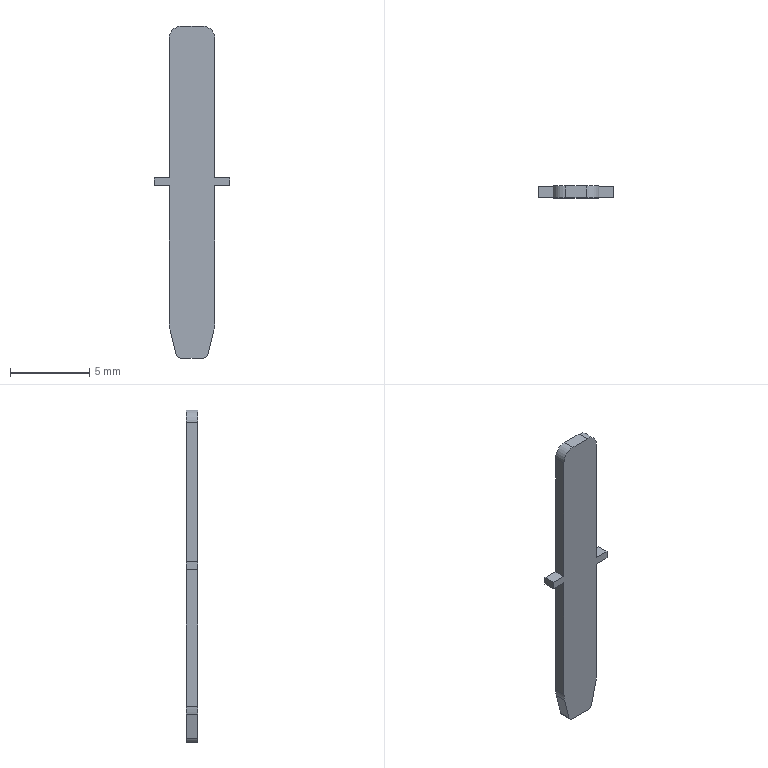Part | SolidWorks | features BaseBody 1 | 1 solid | 22 faces | box 4.8 x 0.75 x 21 mm | volume 45.412 mm3 | plane 16 | cylinder 6 | commonest cylinder face diameters 0.6 x2 1.6 x2 4 x2
STEP:
#1=CARTESIAN_POINT('',(-1.45,0.375,-9.6));
#2=VERTEX_POINT('',#1);
#3=CARTESIAN_POINT('',(-1.45,0.375,-0.8));
#4=VERTEX_POINT('',#3);
#5=CARTESIAN_POINT('',(-1.45,0.375,0.));
#6=DIRECTION('',(0.,0.,1.));
#7=VECTOR('',#6,1000.);
#8=LINE('',#5,#7);
#9=EDGE_CURVE('',#2,#4,#8,.T.);
#10=ORIENTED_EDGE('',*,*,#9,.T.);
#11=CARTESIAN_POINT('',(-0.65,0.375,0.));
#12=VERTEX_POINT('',#11);
#13=CARTESIAN_POINT('',(-0.65,0.375,-0.8));
#14=DIRECTION('',(0.,1.,0.));
#15=DIRECTION('',(0.,0.,-1.));
#16=AXIS2_PLACEMENT_3D('',#13,#14,#15);
#17=CIRCLE('',#16,0.8);
#18=EDGE_CURVE('',#4,#12,#17,.T.);
#19=ORIENTED_EDGE('',*,*,#18,.T.);
#20=CARTESIAN_POINT('',(0.65,0.375,0.));
#21=VERTEX_POINT('',#20);
#22=CARTESIAN_POINT('',(0.,0.375,0.));
#23=DIRECTION('',(1.,0.,0.));
#24=VECTOR('',#23,1000.);
#25=LINE('',#22,#24);
#26=EDGE_CURVE('',#12,#21,#25,.T.);
#27=ORIENTED_EDGE('',*,*,#26,.T.);
#28=CARTESIAN_POINT('',(1.45,0.375,-0.8));
#29=VERTEX_POINT('',#28);
#30=CARTESIAN_POINT('',(0.65,0.375,-0.8));
#31=DIRECTION('',(0.,1.,0.));
#32=DIRECTION('',(0.,0.,-1.));
#33=AXIS2_PLACEMENT_3D('',#30,#31,#32);
#34=CIRCLE('',#33,0.8);
#35=EDGE_CURVE('',#21,#29,#34,.T.);
#36=ORIENTED_EDGE('',*,*,#35,.T.);
#37=CARTESIAN_POINT('',(1.45,0.375,-9.6));
#38=VERTEX_POINT('',#37);
#39=CARTESIAN_POINT('',(1.45,0.375,0.));
#40=DIRECTION('',(0.,0.,-1.));
#41=VECTOR('',#40,1000.);
#42=LINE('',#39,#41);
#43=EDGE_CURVE('',#29,#38,#42,.T.);
#44=ORIENTED_EDGE('',*,*,#43,.T.);
#45=CARTESIAN_POINT('',(2.4,0.375,-9.6));
#46=VERTEX_POINT('',#45);
#47=CARTESIAN_POINT('',(0.,0.375,-9.6));
#48=DIRECTION('',(1.,0.,0.));
#49=VECTOR('',#48,1000.);
#50=LINE('',#47,#49);
#51=EDGE_CURVE('',#38,#46,#50,.T.);
#52=ORIENTED_EDGE('',*,*,#51,.T.);
#53=CARTESIAN_POINT('',(2.4,0.375,-10.1));
#54=VERTEX_POINT('',#53);
#55=CARTESIAN_POINT('',(2.4,0.375,0.));
#56=DIRECTION('',(0.,0.,-1.));
#57=VECTOR('',#56,1000.);
#58=LINE('',#55,#57);
#59=EDGE_CURVE('',#46,#54,#58,.T.);
#60=ORIENTED_EDGE('',*,*,#59,.T.);
#61=CARTESIAN_POINT('',(1.45,0.375,-10.1));
#62=VERTEX_POINT('',#61);
#63=CARTESIAN_POINT('',(0.,0.375,-10.1));
#64=DIRECTION('',(-1.,0.,0.));
#65=VECTOR('',#64,1000.);
#66=LINE('',#63,#65);
#67=EDGE_CURVE('',#54,#62,#66,.T.);
#68=ORIENTED_EDGE('',*,*,#67,.T.);
#69=CARTESIAN_POINT('',(1.45,0.375,-18.754));
#70=VERTEX_POINT('',#69);
#71=CARTESIAN_POINT('',(1.45,0.375,0.));
#72=DIRECTION('',(0.,0.,-1.));
#73=VECTOR('',#72,1000.);
#74=LINE('',#71,#73);
#75=EDGE_CURVE('',#62,#70,#74,.T.);
#76=ORIENTED_EDGE('',*,*,#75,.T.);
#77=CARTESIAN_POINT('',(1.39,0.375,-19.239));
#78=VERTEX_POINT('',#77);
#79=CARTESIAN_POINT('',(-0.55,0.375,-18.754));
#80=DIRECTION('',(0.,1.,0.));
#81=DIRECTION('',(0.,0.,1.));
#82=AXIS2_PLACEMENT_3D('',#79,#80,#81);
#83=CIRCLE('',#82,2.);
#84=EDGE_CURVE('',#70,#78,#83,.T.);
#85=ORIENTED_EDGE('',*,*,#84,.T.);
#86=CARTESIAN_POINT('',(1.007,0.375,-20.773));
#87=VERTEX_POINT('',#86);
#88=CARTESIAN_POINT('',(1.39,0.375,-19.239));
#89=DIRECTION('',(-0.2425,0.,-0.9701));
#90=VECTOR('',#89,1000.);
#91=LINE('',#88,#90);
#92=EDGE_CURVE('',#78,#87,#91,.T.);
#93=ORIENTED_EDGE('',*,*,#92,.T.);
#94=CARTESIAN_POINT('',(0.7158,0.375,-21.));
#95=VERTEX_POINT('',#94);
#96=CARTESIAN_POINT('',(0.7158,0.375,-20.7));
#97=DIRECTION('',(0.,1.,0.));
#98=DIRECTION('',(0.,0.,-1.));
#99=AXIS2_PLACEMENT_3D('',#96,#97,#98);
#100=CIRCLE('',#99,0.3);
#101=EDGE_CURVE('',#87,#95,#100,.T.);
#102=ORIENTED_EDGE('',*,*,#101,.T.);
#103=CARTESIAN_POINT('',(-0.7158,0.375,-21.));
#104=VERTEX_POINT('',#103);
#105=CARTESIAN_POINT('',(0.,0.375,-21.));
#106=DIRECTION('',(-1.,0.,0.));
#107=VECTOR('',#106,1000.);
#108=LINE('',#105,#107);
#109=EDGE_CURVE('',#95,#104,#108,.T.);
#110=ORIENTED_EDGE('',*,*,#109,.T.);
#111=CARTESIAN_POINT('',(-1.007,0.375,-20.773));
#112=VERTEX_POINT('',#111);
#113=CARTESIAN_POINT('',(-0.7158,0.375,-20.7));
#114=DIRECTION('',(0.,1.,0.));
#115=DIRECTION('',(0.,0.,1.));
#116=AXIS2_PLACEMENT_3D('',#113,#114,#115);
#117=CIRCLE('',#116,0.3);
#118=EDGE_CURVE('',#104,#112,#117,.T.);
#119=ORIENTED_EDGE('',*,*,#118,.T.);
#120=CARTESIAN_POINT('',(-1.39,0.375,-19.239));
#121=VERTEX_POINT('',#120);
#122=CARTESIAN_POINT('',(-1.007,0.375,-20.773));
#123=DIRECTION('',(-0.2425,0.,0.9701));
#124=VECTOR('',#123,1000.);
#125=LINE('',#122,#124);
#126=EDGE_CURVE('',#112,#121,#125,.T.);
#127=ORIENTED_EDGE('',*,*,#126,.T.);
#128=CARTESIAN_POINT('',(-1.45,0.375,-18.754));
#129=VERTEX_POINT('',#128);
#130=CARTESIAN_POINT('',(0.55,0.375,-18.754));
#131=DIRECTION('',(0.,1.,0.));
#132=DIRECTION('',(0.,0.,-1.));
#133=AXIS2_PLACEMENT_3D('',#130,#131,#132);
#134=CIRCLE('',#133,2.);
#135=EDGE_CURVE('',#121,#129,#134,.T.);
#136=ORIENTED_EDGE('',*,*,#135,.T.);
#137=CARTESIAN_POINT('',(-1.45,0.375,-10.1));
#138=VERTEX_POINT('',#137);
#139=CARTESIAN_POINT('',(-1.45,0.375,0.));
#140=DIRECTION('',(0.,0.,1.));
#141=VECTOR('',#140,1000.);
#142=LINE('',#139,#141);
#143=EDGE_CURVE('',#129,#138,#142,.T.);
#144=ORIENTED_EDGE('',*,*,#143,.T.);
#145=CARTESIAN_POINT('',(-2.4,0.375,-10.1));
#146=VERTEX_POINT('',#145);
#147=CARTESIAN_POINT('',(0.,0.375,-10.1));
#148=DIRECTION('',(-1.,0.,0.));
#149=VECTOR('',#148,1000.);
#150=LINE('',#147,#149);
#151=EDGE_CURVE('',#138,#146,#150,.T.);
#152=ORIENTED_EDGE('',*,*,#151,.T.);
#153=CARTESIAN_POINT('',(-2.4,0.375,-9.6));
#154=VERTEX_POINT('',#153);
#155=CARTESIAN_POINT('',(-2.4,0.375,0.));
#156=DIRECTION('',(0.,0.,1.));
#157=VECTOR('',#156,1000.);
#158=LINE('',#155,#157);
#159=EDGE_CURVE('',#146,#154,#158,.T.);
#160=ORIENTED_EDGE('',*,*,#159,.T.);
#161=CARTESIAN_POINT('',(0.,0.375,-9.6));
#162=DIRECTION('',(1.,0.,0.));
#163=VECTOR('',#162,1000.);
#164=LINE('',#161,#163);
#165=EDGE_CURVE('',#154,#2,#164,.T.);
#166=ORIENTED_EDGE('',*,*,#165,.T.);
#167=EDGE_LOOP('',(#10,#19,#27,#36,#44,#52,#60,#68,#76,#85,#93,#102,#110,#119,#127,#136,#144,#152,#160,#166));
#168=FACE_OUTER_BOUND('',#167,.T.);
#169=CARTESIAN_POINT('',(0.,0.375,0.));
#170=DIRECTION('',(0.,1.,0.));
#171=DIRECTION('',(0.,0.,1.));
#172=AXIS2_PLACEMENT_3D('',#169,#170,#171);
#173=PLANE('',#172);
#174=ADVANCED_FACE('',(#168),#173,.T.);
#175=CARTESIAN_POINT('',(-1.45,-0.375,-0.8));
#176=VERTEX_POINT('',#175);
#177=CARTESIAN_POINT('',(-1.45,1.413,-0.8));
#178=DIRECTION('',(0.,-1.,0.));
#179=VECTOR('',#178,1000.);
#180=LINE('',#177,#179);
#181=EDGE_CURVE('',#4,#176,#180,.T.);
#182=ORIENTED_EDGE('',*,*,#181,.T.);
#183=CARTESIAN_POINT('',(-0.65,-0.375,0.));
#184=VERTEX_POINT('',#183);
#185=CARTESIAN_POINT('',(-0.65,-0.375,-0.8));
#186=DIRECTION('',(0.,1.,0.));
#187=DIRECTION('',(0.,0.,-1.));
#188=AXIS2_PLACEMENT_3D('',#185,#186,#187);
#189=CIRCLE('',#188,0.8);
#190=EDGE_CURVE('',#176,#184,#189,.T.);
#191=ORIENTED_EDGE('',*,*,#190,.T.);
#192=CARTESIAN_POINT('',(-0.65,1.413,0.));
#193=DIRECTION('',(0.,1.,0.));
#194=VECTOR('',#193,1000.);
#195=LINE('',#192,#194);
#196=EDGE_CURVE('',#184,#12,#195,.T.);
#197=ORIENTED_EDGE('',*,*,#196,.T.);
#198=ORIENTED_EDGE('',*,*,#18,.F.);
#199=EDGE_LOOP('',(#182,#191,#197,#198));
#200=FACE_OUTER_BOUND('',#199,.T.);
#201=CARTESIAN_POINT('',(-0.65,1.413,-0.8));
#202=DIRECTION('',(0.,-1.,0.));
#203=DIRECTION('',(0.,0.,-1.));
#204=AXIS2_PLACEMENT_3D('',#201,#202,#203);
#205=CYLINDRICAL_SURFACE('',#204,0.8);
#206=ADVANCED_FACE('',(#200),#205,.T.);
#207=CARTESIAN_POINT('',(-1.45,-0.375,-9.6));
#208=VERTEX_POINT('',#207);
#209=CARTESIAN_POINT('',(-1.45,-0.375,-21.));
#210=DIRECTION('',(0.,0.,1.));
#211=VECTOR('',#210,1000.);
#212=LINE('',#209,#211);
#213=EDGE_CURVE('',#208,#176,#212,.T.);
#214=ORIENTED_EDGE('',*,*,#213,.T.);
#215=ORIENTED_EDGE('',*,*,#181,.F.);
#216=ORIENTED_EDGE('',*,*,#9,.F.);
#217=CARTESIAN_POINT('',(-1.45,-0.375,-9.6));
#218=DIRECTION('',(0.,-1.,0.));
#219=VECTOR('',#218,1000.);
#220=LINE('',#217,#219);
#221=EDGE_CURVE('',#2,#208,#220,.T.);
#222=ORIENTED_EDGE('',*,*,#221,.T.);
#223=EDGE_LOOP('',(#214,#215,#216,#222));
#224=FACE_OUTER_BOUND('',#223,.T.);
#225=CARTESIAN_POINT('',(-1.45,-0.375,-21.));
#226=DIRECTION('',(-1.,0.,0.));
#227=DIRECTION('',(0.,0.,1.));
#228=AXIS2_PLACEMENT_3D('',#225,#226,#227);
#229=PLANE('',#228);
#230=ADVANCED_FACE('',(#224),#229,.T.);
#231=CARTESIAN_POINT('',(-2.4,-0.375,-9.6));
#232=VERTEX_POINT('',#231);
#233=CARTESIAN_POINT('',(-2.4,-0.375,-9.6));
#234=DIRECTION('',(1.,0.,0.));
#235=VECTOR('',#234,1000.);
#236=LINE('',#233,#235);
#237=EDGE_CURVE('',#232,#208,#236,.T.);
#238=ORIENTED_EDGE('',*,*,#237,.T.);
#239=ORIENTED_EDGE('',*,*,#221,.F.);
#240=ORIENTED_EDGE('',*,*,#165,.F.);
#241=CARTESIAN_POINT('',(-2.4,0.375,-9.6));
#242=DIRECTION('',(0.,-1.,0.));
#243=VECTOR('',#242,1000.);
#244=LINE('',#241,#243);
#245=EDGE_CURVE('',#154,#232,#244,.T.);
#246=ORIENTED_EDGE('',*,*,#245,.T.);
#247=EDGE_LOOP('',(#238,#239,#240,#246));
#248=FACE_OUTER_BOUND('',#247,.T.);
#249=CARTESIAN_POINT('',(-2.4,0.375,-9.6));
#250=DIRECTION('',(0.,0.,1.));
#251=DIRECTION('',(1.,0.,0.));
#252=AXIS2_PLACEMENT_3D('',#249,#250,#251);
#253=PLANE('',#252);
#254=ADVANCED_FACE('',(#248),#253,.T.);
#255=ORIENTED_EDGE('',*,*,#245,.F.);
#256=ORIENTED_EDGE('',*,*,#159,.F.);
#257=CARTESIAN_POINT('',(-2.4,-0.375,-10.1));
#258=VERTEX_POINT('',#257);
#259=CARTESIAN_POINT('',(-2.4,0.375,-10.1));
#260=DIRECTION('',(0.,-1.,0.));
#261=VECTOR('',#260,1000.);
#262=LINE('',#259,#261);
#263=EDGE_CURVE('',#146,#258,#262,.T.);
#264=ORIENTED_EDGE('',*,*,#263,.T.);
#265=CARTESIAN_POINT('',(-2.4,-0.375,-10.1));
#266=DIRECTION('',(0.,0.,1.));
#267=VECTOR('',#266,1000.);
#268=LINE('',#265,#267);
#269=EDGE_CURVE('',#258,#232,#268,.T.);
#270=ORIENTED_EDGE('',*,*,#269,.T.);
#271=EDGE_LOOP('',(#255,#256,#264,#270));
#272=FACE_OUTER_BOUND('',#271,.T.);
#273=CARTESIAN_POINT('',(-2.4,0.375,-10.1));
#274=DIRECTION('',(-1.,0.,0.));
#275=DIRECTION('',(0.,0.,1.));
#276=AXIS2_PLACEMENT_3D('',#273,#274,#275);
#277=PLANE('',#276);
#278=ADVANCED_FACE('',(#272),#277,.T.);
#279=ORIENTED_EDGE('',*,*,#151,.F.);
#280=CARTESIAN_POINT('',(-1.45,-0.375,-10.1));
#281=VERTEX_POINT('',#280);
#282=CARTESIAN_POINT('',(-1.45,0.375,-10.1));
#283=DIRECTION('',(0.,-1.,0.));
#284=VECTOR('',#283,1000.);
#285=LINE('',#282,#284);
#286=EDGE_CURVE('',#138,#281,#285,.T.);
#287=ORIENTED_EDGE('',*,*,#286,.T.);
#288=CARTESIAN_POINT('',(2.4,-0.375,-10.1));
#289=DIRECTION('',(-1.,0.,0.));
#290=VECTOR('',#289,1000.);
#291=LINE('',#288,#290);
#292=EDGE_CURVE('',#281,#258,#291,.T.);
#293=ORIENTED_EDGE('',*,*,#292,.T.);
#294=ORIENTED_EDGE('',*,*,#263,.F.);
#295=EDGE_LOOP('',(#279,#287,#293,#294));
#296=FACE_OUTER_BOUND('',#295,.T.);
#297=CARTESIAN_POINT('',(2.4,0.375,-10.1));
#298=DIRECTION('',(0.,0.,-1.));
#299=DIRECTION('',(-1.,0.,0.));
#300=AXIS2_PLACEMENT_3D('',#297,#298,#299);
#301=PLANE('',#300);
#302=ADVANCED_FACE('',(#296),#301,.T.);
#303=ORIENTED_EDGE('',*,*,#143,.F.);
#304=CARTESIAN_POINT('',(-1.45,-0.375,-18.754));
#305=VERTEX_POINT('',#304);
#306=CARTESIAN_POINT('',(-1.45,-0.375,-18.754));
#307=DIRECTION('',(0.,-1.,0.));
#308=VECTOR('',#307,1000.);
#309=LINE('',#306,#308);
#310=EDGE_CURVE('',#129,#305,#309,.T.);
#311=ORIENTED_EDGE('',*,*,#310,.T.);
#312=CARTESIAN_POINT('',(-1.45,-0.375,-21.));
#313=DIRECTION('',(0.,0.,1.));
#314=VECTOR('',#313,1000.);
#315=LINE('',#312,#314);
#316=EDGE_CURVE('',#305,#281,#315,.T.);
#317=ORIENTED_EDGE('',*,*,#316,.T.);
#318=ORIENTED_EDGE('',*,*,#286,.F.);
#319=EDGE_LOOP('',(#303,#311,#317,#318));
#320=FACE_OUTER_BOUND('',#319,.T.);
#321=CARTESIAN_POINT('',(-1.45,-0.375,-21.));
#322=DIRECTION('',(-1.,0.,0.));
#323=DIRECTION('',(0.,0.,1.));
#324=AXIS2_PLACEMENT_3D('',#321,#322,#323);
#325=PLANE('',#324);
#326=ADVANCED_FACE('',(#320),#325,.T.);
#327=CARTESIAN_POINT('',(-1.39,-0.375,-19.239));
#328=VERTEX_POINT('',#327);
#329=CARTESIAN_POINT('',(-1.39,2.856,-19.239));
#330=DIRECTION('',(0.,-1.,0.));
#331=VECTOR('',#330,1000.);
#332=LINE('',#329,#331);
#333=EDGE_CURVE('',#121,#328,#332,.T.);
#334=ORIENTED_EDGE('',*,*,#333,.T.);
#335=CARTESIAN_POINT('',(0.55,-0.375,-18.754));
#336=DIRECTION('',(0.,1.,0.));
#337=DIRECTION('',(0.,0.,-1.));
#338=AXIS2_PLACEMENT_3D('',#335,#336,#337);
#339=CIRCLE('',#338,2.);
#340=EDGE_CURVE('',#328,#305,#339,.T.);
#341=ORIENTED_EDGE('',*,*,#340,.T.);
#342=ORIENTED_EDGE('',*,*,#310,.F.);
#343=ORIENTED_EDGE('',*,*,#135,.F.);
#344=EDGE_LOOP('',(#334,#341,#342,#343));
#345=FACE_OUTER_BOUND('',#344,.T.);
#346=CARTESIAN_POINT('',(0.55,2.856,-18.754));
#347=DIRECTION('',(0.,-1.,0.));
#348=DIRECTION('',(0.,0.,-1.));
#349=AXIS2_PLACEMENT_3D('',#346,#347,#348);
#350=CYLINDRICAL_SURFACE('',#349,2.);
#351=ADVANCED_FACE('',(#345),#350,.T.);
#352=ORIENTED_EDGE('',*,*,#126,.F.);
#353=CARTESIAN_POINT('',(-1.007,-0.375,-20.773));
#354=VERTEX_POINT('',#353);
#355=CARTESIAN_POINT('',(-1.007,0.,-20.773));
#356=DIRECTION('',(0.,-1.,0.));
#357=VECTOR('',#356,1000.);
#358=LINE('',#355,#357);
#359=EDGE_CURVE('',#112,#354,#358,.T.);
#360=ORIENTED_EDGE('',*,*,#359,.T.);
#361=CARTESIAN_POINT('',(-1.2,-0.375,-20.));
#362=DIRECTION('',(-0.2425,0.,0.9701));
#363=VECTOR('',#362,1000.);
#364=LINE('',#361,#363);
#365=EDGE_CURVE('',#354,#328,#364,.T.);
#366=ORIENTED_EDGE('',*,*,#365,.T.);
#367=ORIENTED_EDGE('',*,*,#333,.F.);
#368=EDGE_LOOP('',(#352,#360,#366,#367));
#369=FACE_OUTER_BOUND('',#368,.T.);
#370=CARTESIAN_POINT('',(-1.2,0.,-20.));
#371=DIRECTION('',(-0.9701,0.,-0.2425));
#372=DIRECTION('',(-0.2425,0.,0.9701));
#373=AXIS2_PLACEMENT_3D('',#370,#371,#372);
#374=PLANE('',#373);
#375=ADVANCED_FACE('',(#369),#374,.T.);
#376=ORIENTED_EDGE('',*,*,#359,.F.);
#377=ORIENTED_EDGE('',*,*,#118,.F.);
#378=CARTESIAN_POINT('',(-0.7158,-0.375,-21.));
#379=VERTEX_POINT('',#378);
#380=CARTESIAN_POINT('',(-0.7158,-1.353,-21.));
#381=DIRECTION('',(0.,-1.,0.));
#382=VECTOR('',#381,1000.);
#383=LINE('',#380,#382);
#384=EDGE_CURVE('',#104,#379,#383,.T.);
#385=ORIENTED_EDGE('',*,*,#384,.T.);
#386=CARTESIAN_POINT('',(-0.7158,-0.375,-20.7));
#387=DIRECTION('',(0.,1.,0.));
#388=DIRECTION('',(0.,0.,1.));
#389=AXIS2_PLACEMENT_3D('',#386,#387,#388);
#390=CIRCLE('',#389,0.3);
#391=EDGE_CURVE('',#379,#354,#390,.T.);
#392=ORIENTED_EDGE('',*,*,#391,.T.);
#393=EDGE_LOOP('',(#376,#377,#385,#392));
#394=FACE_OUTER_BOUND('',#393,.T.);
#395=CARTESIAN_POINT('',(-0.7158,-1.353,-20.7));
#396=DIRECTION('',(0.,1.,0.));
#397=DIRECTION('',(0.,0.,1.));
#398=AXIS2_PLACEMENT_3D('',#395,#396,#397);
#399=CYLINDRICAL_SURFACE('',#398,0.3);
#400=ADVANCED_FACE('',(#394),#399,.T.);
#401=ORIENTED_EDGE('',*,*,#109,.F.);
#402=CARTESIAN_POINT('',(0.7158,-0.375,-21.));
#403=VERTEX_POINT('',#402);
#404=CARTESIAN_POINT('',(0.7158,-0.375,-21.));
#405=DIRECTION('',(0.,-1.,0.));
#406=VECTOR('',#405,1000.);
#407=LINE('',#404,#406);
#408=EDGE_CURVE('',#95,#403,#407,.T.);
#409=ORIENTED_EDGE('',*,*,#408,.T.);
#410=CARTESIAN_POINT('',(1.45,-0.375,-21.));
#411=DIRECTION('',(-1.,0.,0.));
#412=VECTOR('',#411,1000.);
#413=LINE('',#410,#412);
#414=EDGE_CURVE('',#403,#379,#413,.T.);
#415=ORIENTED_EDGE('',*,*,#414,.T.);
#416=ORIENTED_EDGE('',*,*,#384,.F.);
#417=EDGE_LOOP('',(#401,#409,#415,#416));
#418=FACE_OUTER_BOUND('',#417,.T.);
#419=CARTESIAN_POINT('',(1.45,-0.375,-21.));
#420=DIRECTION('',(0.,0.,-1.));
#421=DIRECTION('',(-1.,0.,0.));
#422=AXIS2_PLACEMENT_3D('',#419,#420,#421);
#423=PLANE('',#422);
#424=ADVANCED_FACE('',(#418),#423,.T.);
#425=CARTESIAN_POINT('',(1.007,-0.375,-20.773));
#426=VERTEX_POINT('',#425);
#427=CARTESIAN_POINT('',(1.007,1.353,-20.773));
#428=DIRECTION('',(0.,-1.,0.));
#429=VECTOR('',#428,1000.);
#430=LINE('',#427,#429);
#431=EDGE_CURVE('',#87,#426,#430,.T.);
#432=ORIENTED_EDGE('',*,*,#431,.T.);
#433=CARTESIAN_POINT('',(0.7158,-0.375,-20.7));
#434=DIRECTION('',(0.,1.,0.));
#435=DIRECTION('',(0.,0.,-1.));
#436=AXIS2_PLACEMENT_3D('',#433,#434,#435);
#437=CIRCLE('',#436,0.3);
#438=EDGE_CURVE('',#426,#403,#437,.T.);
#439=ORIENTED_EDGE('',*,*,#438,.T.);
#440=ORIENTED_EDGE('',*,*,#408,.F.);
#441=ORIENTED_EDGE('',*,*,#101,.F.);
#442=EDGE_LOOP('',(#432,#439,#440,#441));
#443=FACE_OUTER_BOUND('',#442,.T.);
#444=CARTESIAN_POINT('',(0.7158,1.353,-20.7));
#445=DIRECTION('',(0.,-1.,0.));
#446=DIRECTION('',(0.,0.,-1.));
#447=AXIS2_PLACEMENT_3D('',#444,#445,#446);
#448=CYLINDRICAL_SURFACE('',#447,0.3);
#449=ADVANCED_FACE('',(#443),#448,.T.);
#450=CARTESIAN_POINT('',(1.39,-0.375,-19.239));
#451=VERTEX_POINT('',#450);
#452=CARTESIAN_POINT('',(1.2,-0.375,-20.));
#453=DIRECTION('',(-0.2425,0.,-0.9701));
#454=VECTOR('',#453,1000.);
#455=LINE('',#452,#454);
#456=EDGE_CURVE('',#451,#426,#455,.T.);
#457=ORIENTED_EDGE('',*,*,#456,.T.);
#458=ORIENTED_EDGE('',*,*,#431,.F.);
#459=ORIENTED_EDGE('',*,*,#92,.F.);
#460=CARTESIAN_POINT('',(1.39,0.,-19.239));
#461=DIRECTION('',(0.,-1.,0.));
#462=VECTOR('',#461,1000.);
#463=LINE('',#460,#462);
#464=EDGE_CURVE('',#78,#451,#463,.T.);
#465=ORIENTED_EDGE('',*,*,#464,.T.);
#466=EDGE_LOOP('',(#457,#458,#459,#465));
#467=FACE_OUTER_BOUND('',#466,.T.);
#468=CARTESIAN_POINT('',(1.2,0.,-20.));
#469=DIRECTION('',(0.9701,0.,-0.2425));
#470=DIRECTION('',(-0.2425,0.,-0.9701));
#471=AXIS2_PLACEMENT_3D('',#468,#469,#470);
#472=PLANE('',#471);
#473=ADVANCED_FACE('',(#467),#472,.T.);
#474=ORIENTED_EDGE('',*,*,#464,.F.);
#475=ORIENTED_EDGE('',*,*,#84,.F.);
#476=CARTESIAN_POINT('',(1.45,-0.375,-18.754));
#477=VERTEX_POINT('',#476);
#478=CARTESIAN_POINT('',(1.45,-2.856,-18.754));
#479=DIRECTION('',(0.,-1.,0.));
#480=VECTOR('',#479,1000.);
#481=LINE('',#478,#480);
#482=EDGE_CURVE('',#70,#477,#481,.T.);
#483=ORIENTED_EDGE('',*,*,#482,.T.);
#484=CARTESIAN_POINT('',(-0.55,-0.375,-18.754));
#485=DIRECTION('',(0.,1.,0.));
#486=DIRECTION('',(0.,0.,1.));
#487=AXIS2_PLACEMENT_3D('',#484,#485,#486);
#488=CIRCLE('',#487,2.);
#489=EDGE_CURVE('',#477,#451,#488,.T.);
#490=ORIENTED_EDGE('',*,*,#489,.T.);
#491=EDGE_LOOP('',(#474,#475,#483,#490));
#492=FACE_OUTER_BOUND('',#491,.T.);
#493=CARTESIAN_POINT('',(-0.55,-2.856,-18.754));
#494=DIRECTION('',(0.,1.,0.));
#495=DIRECTION('',(0.,0.,1.));
#496=AXIS2_PLACEMENT_3D('',#493,#494,#495);
#497=CYLINDRICAL_SURFACE('',#496,2.);
#498=ADVANCED_FACE('',(#492),#497,.T.);
#499=CARTESIAN_POINT('',(1.45,-0.375,-10.1));
#500=VERTEX_POINT('',#499);
#501=CARTESIAN_POINT('',(1.45,-0.375,0.));
#502=DIRECTION('',(0.,0.,-1.));
#503=VECTOR('',#502,1000.);
#504=LINE('',#501,#503);
#505=EDGE_CURVE('',#500,#477,#504,.T.);
#506=ORIENTED_EDGE('',*,*,#505,.T.);
#507=ORIENTED_EDGE('',*,*,#482,.F.);
#508=ORIENTED_EDGE('',*,*,#75,.F.);
#509=CARTESIAN_POINT('',(1.45,-0.375,-10.1));
#510=DIRECTION('',(0.,-1.,0.));
#511=VECTOR('',#510,1000.);
#512=LINE('',#509,#511);
#513=EDGE_CURVE('',#62,#500,#512,.T.);
#514=ORIENTED_EDGE('',*,*,#513,.T.);
#515=EDGE_LOOP('',(#506,#507,#508,#514));
#516=FACE_OUTER_BOUND('',#515,.T.);
#517=CARTESIAN_POINT('',(1.45,-0.375,0.));
#518=DIRECTION('',(1.,0.,0.));
#519=DIRECTION('',(0.,0.,-1.));
#520=AXIS2_PLACEMENT_3D('',#517,#518,#519);
#521=PLANE('',#520);
#522=ADVANCED_FACE('',(#516),#521,.T.);
#523=CARTESIAN_POINT('',(2.4,-0.375,-10.1));
#524=VERTEX_POINT('',#523);
#525=CARTESIAN_POINT('',(2.4,-0.375,-10.1));
#526=DIRECTION('',(-1.,0.,0.));
#527=VECTOR('',#526,1000.);
#528=LINE('',#525,#527);
#529=EDGE_CURVE('',#524,#500,#528,.T.);
#530=ORIENTED_EDGE('',*,*,#529,.T.);
#531=ORIENTED_EDGE('',*,*,#513,.F.);
#532=ORIENTED_EDGE('',*,*,#67,.F.);
#533=CARTESIAN_POINT('',(2.4,0.375,-10.1));
#534=DIRECTION('',(0.,-1.,0.));
#535=VECTOR('',#534,1000.);
#536=LINE('',#533,#535);
#537=EDGE_CURVE('',#54,#524,#536,.T.);
#538=ORIENTED_EDGE('',*,*,#537,.T.);
#539=EDGE_LOOP('',(#530,#531,#532,#538));
#540=FACE_OUTER_BOUND('',#539,.T.);
#541=CARTESIAN_POINT('',(2.4,0.375,-10.1));
#542=DIRECTION('',(0.,0.,-1.));
#543=DIRECTION('',(-1.,0.,0.));
#544=AXIS2_PLACEMENT_3D('',#541,#542,#543);
#545=PLANE('',#544);
#546=ADVANCED_FACE('',(#540),#545,.T.);
#547=ORIENTED_EDGE('',*,*,#537,.F.);
#548=ORIENTED_EDGE('',*,*,#59,.F.);
#549=CARTESIAN_POINT('',(2.4,-0.375,-9.6));
#550=VERTEX_POINT('',#549);
#551=CARTESIAN_POINT('',(2.4,0.375,-9.6));
#552=DIRECTION('',(0.,-1.,0.));
#553=VECTOR('',#552,1000.);
#554=LINE('',#551,#553);
#555=EDGE_CURVE('',#46,#550,#554,.T.);
#556=ORIENTED_EDGE('',*,*,#555,.T.);
#557=CARTESIAN_POINT('',(2.4,-0.375,-9.6));
#558=DIRECTION('',(0.,0.,-1.));
#559=VECTOR('',#558,1000.);
#560=LINE('',#557,#559);
#561=EDGE_CURVE('',#550,#524,#560,.T.);
#562=ORIENTED_EDGE('',*,*,#561,.T.);
#563=EDGE_LOOP('',(#547,#548,#556,#562));
#564=FACE_OUTER_BOUND('',#563,.T.);
#565=CARTESIAN_POINT('',(2.4,0.375,-9.6));
#566=DIRECTION('',(1.,0.,0.));
#567=DIRECTION('',(0.,0.,-1.));
#568=AXIS2_PLACEMENT_3D('',#565,#566,#567);
#569=PLANE('',#568);
#570=ADVANCED_FACE('',(#564),#569,.T.);
#571=ORIENTED_EDGE('',*,*,#51,.F.);
#572=CARTESIAN_POINT('',(1.45,-0.375,-9.6));
#573=VERTEX_POINT('',#572);
#574=CARTESIAN_POINT('',(1.45,0.375,-9.6));
#575=DIRECTION('',(0.,-1.,0.));
#576=VECTOR('',#575,1000.);
#577=LINE('',#574,#576);
#578=EDGE_CURVE('',#38,#573,#577,.T.);
#579=ORIENTED_EDGE('',*,*,#578,.T.);
#580=CARTESIAN_POINT('',(-2.4,-0.375,-9.6));
#581=DIRECTION('',(1.,0.,0.));
#582=VECTOR('',#581,1000.);
#583=LINE('',#580,#582);
#584=EDGE_CURVE('',#573,#550,#583,.T.);
#585=ORIENTED_EDGE('',*,*,#584,.T.);
#586=ORIENTED_EDGE('',*,*,#555,.F.);
#587=EDGE_LOOP('',(#571,#579,#585,#586));
#588=FACE_OUTER_BOUND('',#587,.T.);
#589=CARTESIAN_POINT('',(-2.4,0.375,-9.6));
#590=DIRECTION('',(0.,0.,1.));
#591=DIRECTION('',(1.,0.,0.));
#592=AXIS2_PLACEMENT_3D('',#589,#590,#591);
#593=PLANE('',#592);
#594=ADVANCED_FACE('',(#588),#593,.T.);
#595=ORIENTED_EDGE('',*,*,#43,.F.);
#596=CARTESIAN_POINT('',(1.45,-0.375,-0.8));
#597=VERTEX_POINT('',#596);
#598=CARTESIAN_POINT('',(1.45,-0.375,-0.8));
#599=DIRECTION('',(0.,-1.,0.));
#600=VECTOR('',#599,1000.);
#601=LINE('',#598,#600);
#602=EDGE_CURVE('',#29,#597,#601,.T.);
#603=ORIENTED_EDGE('',*,*,#602,.T.);
#604=CARTESIAN_POINT('',(1.45,-0.375,0.));
#605=DIRECTION('',(0.,0.,-1.));
#606=VECTOR('',#605,1000.);
#607=LINE('',#604,#606);
#608=EDGE_CURVE('',#597,#573,#607,.T.);
#609=ORIENTED_EDGE('',*,*,#608,.T.);
#610=ORIENTED_EDGE('',*,*,#578,.F.);
#611=EDGE_LOOP('',(#595,#603,#609,#610));
#612=FACE_OUTER_BOUND('',#611,.T.);
#613=CARTESIAN_POINT('',(1.45,-0.375,0.));
#614=DIRECTION('',(1.,0.,0.));
#615=DIRECTION('',(0.,0.,-1.));
#616=AXIS2_PLACEMENT_3D('',#613,#614,#615);
#617=PLANE('',#616);
#618=ADVANCED_FACE('',(#612),#617,.T.);
#619=CARTESIAN_POINT('',(0.65,-0.375,0.));
#620=VERTEX_POINT('',#619);
#621=CARTESIAN_POINT('',(0.65,1.413,0.));
#622=DIRECTION('',(0.,-1.,0.));
#623=VECTOR('',#622,1000.);
#624=LINE('',#621,#623);
#625=EDGE_CURVE('',#21,#620,#624,.T.);
#626=ORIENTED_EDGE('',*,*,#625,.T.);
#627=CARTESIAN_POINT('',(0.65,-0.375,-0.8));
#628=DIRECTION('',(0.,1.,0.));
#629=DIRECTION('',(0.,0.,-1.));
#630=AXIS2_PLACEMENT_3D('',#627,#628,#629);
#631=CIRCLE('',#630,0.8);
#632=EDGE_CURVE('',#620,#597,#631,.T.);
#633=ORIENTED_EDGE('',*,*,#632,.T.);
#634=ORIENTED_EDGE('',*,*,#602,.F.);
#635=ORIENTED_EDGE('',*,*,#35,.F.);
#636=EDGE_LOOP('',(#626,#633,#634,#635));
#637=FACE_OUTER_BOUND('',#636,.T.);
#638=CARTESIAN_POINT('',(0.65,1.413,-0.8));
#639=DIRECTION('',(0.,-1.,0.));
#640=DIRECTION('',(0.,0.,-1.));
#641=AXIS2_PLACEMENT_3D('',#638,#639,#640);
#642=CYLINDRICAL_SURFACE('',#641,0.8);
#643=ADVANCED_FACE('',(#637),#642,.T.);
#644=ORIENTED_EDGE('',*,*,#26,.F.);
#645=ORIENTED_EDGE('',*,*,#196,.F.);
#646=CARTESIAN_POINT('',(-1.45,-0.375,0.));
#647=DIRECTION('',(1.,0.,0.));
#648=VECTOR('',#647,1000.);
#649=LINE('',#646,#648);
#650=EDGE_CURVE('',#184,#620,#649,.T.);
#651=ORIENTED_EDGE('',*,*,#650,.T.);
#652=ORIENTED_EDGE('',*,*,#625,.F.);
#653=EDGE_LOOP('',(#644,#645,#651,#652));
#654=FACE_OUTER_BOUND('',#653,.T.);
#655=CARTESIAN_POINT('',(-1.45,-0.375,0.));
#656=DIRECTION('',(0.,0.,1.));
#657=DIRECTION('',(1.,0.,0.));
#658=AXIS2_PLACEMENT_3D('',#655,#656,#657);
#659=PLANE('',#658);
#660=ADVANCED_FACE('',(#654),#659,.T.);
#661=ORIENTED_EDGE('',*,*,#237,.F.);
#662=ORIENTED_EDGE('',*,*,#269,.F.);
#663=ORIENTED_EDGE('',*,*,#292,.F.);
#664=ORIENTED_EDGE('',*,*,#316,.F.);
#665=ORIENTED_EDGE('',*,*,#340,.F.);
#666=ORIENTED_EDGE('',*,*,#365,.F.);
#667=ORIENTED_EDGE('',*,*,#391,.F.);
#668=ORIENTED_EDGE('',*,*,#414,.F.);
#669=ORIENTED_EDGE('',*,*,#438,.F.);
#670=ORIENTED_EDGE('',*,*,#456,.F.);
#671=ORIENTED_EDGE('',*,*,#489,.F.);
#672=ORIENTED_EDGE('',*,*,#505,.F.);
#673=ORIENTED_EDGE('',*,*,#529,.F.);
#674=ORIENTED_EDGE('',*,*,#561,.F.);
#675=ORIENTED_EDGE('',*,*,#584,.F.);
#676=ORIENTED_EDGE('',*,*,#608,.F.);
#677=ORIENTED_EDGE('',*,*,#632,.F.);
#678=ORIENTED_EDGE('',*,*,#650,.F.);
#679=ORIENTED_EDGE('',*,*,#190,.F.);
#680=ORIENTED_EDGE('',*,*,#213,.F.);
#681=EDGE_LOOP('',(#661,#662,#663,#664,#665,#666,#667,#668,#669,#670,#671,#672,#673,#674,#675,#676,#677,#678,#679,#680));
#682=FACE_OUTER_BOUND('',#681,.T.);
#683=CARTESIAN_POINT('',(0.,-0.375,0.));
#684=DIRECTION('',(0.,1.,0.));
#685=DIRECTION('',(0.,0.,1.));
#686=AXIS2_PLACEMENT_3D('',#683,#684,#685);
#687=PLANE('',#686);
#688=ADVANCED_FACE('',(#682),#687,.F.);
#689=CLOSED_SHELL('',(#174,#206,#230,#254,#278,#302,#326,#351,#375,#400,#424,#449,#473,#498,#522,#546,#570,#594,#618,#643,#660,#688));
#690=MANIFOLD_SOLID_BREP('',#689);
#691=CARTESIAN_POINT('',(0.,0.,0.));
#692=DIRECTION('',(0.,0.,1.));
#693=DIRECTION('',(1.,0.,0.));
#694=AXIS2_PLACEMENT_3D('',#691,#692,#693);
#695=(LENGTH_UNIT()NAMED_UNIT(*)SI_UNIT(.MILLI.,.METRE.));
#696=UNCERTAINTY_MEASURE_WITH_UNIT(LENGTH_MEASURE(0.00001),#695,'','');
#697=(NAMED_UNIT(*)PLANE_ANGLE_UNIT()SI_UNIT($,.RADIAN.));
#698=(NAMED_UNIT(*)SI_UNIT($,.STERADIAN.)SOLID_ANGLE_UNIT());
#699=(GEOMETRIC_REPRESENTATION_CONTEXT(3)GLOBAL_UNCERTAINTY_ASSIGNED_CONTEXT((#696))GLOBAL_UNIT_ASSIGNED_CONTEXT((#695,#697,#698))REPRESENTATION_CONTEXT('',''));
#700=ADVANCED_BREP_SHAPE_REPRESENTATION('',(#690,#694),#699);